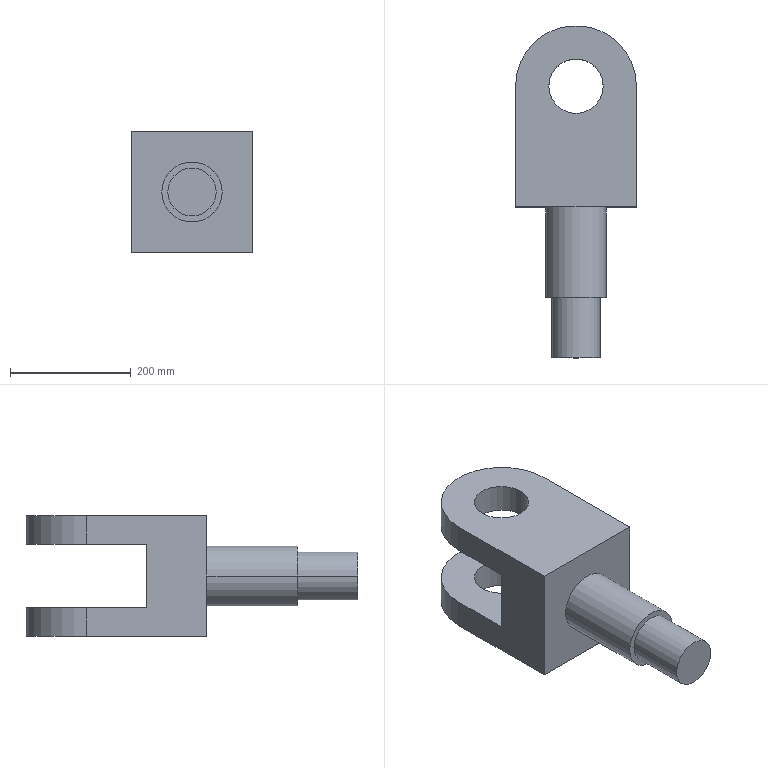Part | SolidWorks | features ICE 4, Extrusion 1 | 1 solid | 20 faces | box 200 x 550 x 200 mm | volume 8468645 mm3 | cylinder 10 | plane 10 | commonest cylinder face diameters 90 x4 80 x2 100 x2 200 x2
STEP:
#1=CARTESIAN_POINT('',(80.402,-409.598,100.));
#2=VERTEX_POINT('',#1);
#3=CARTESIAN_POINT('',(0.4025,-409.598,100.));
#4=VERTEX_POINT('',#3);
#5=CARTESIAN_POINT('',(40.402,-409.598,100.));
#6=DIRECTION('',(0.,-1.,0.));
#7=DIRECTION('',(1.,0.,0.));
#8=AXIS2_PLACEMENT_3D('',#5,#6,#7);
#9=CIRCLE('',#8,40.);
#10=EDGE_CURVE('',#2,#4,#9,.T.);
#11=ORIENTED_EDGE('',*,*,#10,.F.);
#12=CARTESIAN_POINT('',(80.402,-309.598,100.));
#13=VERTEX_POINT('',#12);
#14=CARTESIAN_POINT('',(80.402,-409.598,100.));
#15=DIRECTION('',(0.,1.,0.));
#16=VECTOR('',#15,1000.);
#17=LINE('',#14,#16);
#18=EDGE_CURVE('',#2,#13,#17,.T.);
#19=ORIENTED_EDGE('',*,*,#18,.T.);
#20=CARTESIAN_POINT('',(0.4025,-309.598,100.));
#21=VERTEX_POINT('',#20);
#22=CARTESIAN_POINT('',(40.402,-309.598,100.));
#23=DIRECTION('',(0.,-1.,0.));
#24=DIRECTION('',(1.,0.,0.));
#25=AXIS2_PLACEMENT_3D('',#22,#23,#24);
#26=CIRCLE('',#25,40.);
#27=EDGE_CURVE('',#13,#21,#26,.T.);
#28=ORIENTED_EDGE('',*,*,#27,.T.);
#29=CARTESIAN_POINT('',(0.4025,-409.598,100.));
#30=DIRECTION('',(0.,1.,0.));
#31=VECTOR('',#30,1000.);
#32=LINE('',#29,#31);
#33=EDGE_CURVE('',#4,#21,#32,.T.);
#34=ORIENTED_EDGE('',*,*,#33,.F.);
#35=EDGE_LOOP('',(#11,#19,#28,#34));
#36=FACE_OUTER_BOUND('',#35,.T.);
#37=CARTESIAN_POINT('',(40.402,-409.598,100.));
#38=DIRECTION('',(0.,1.,0.));
#39=DIRECTION('',(-1.,0.,0.));
#40=AXIS2_PLACEMENT_3D('',#37,#38,#39);
#41=CYLINDRICAL_SURFACE('',#40,40.);
#42=ADVANCED_FACE('',(#36),#41,.T.);
#43=CARTESIAN_POINT('',(90.402,-309.598,100.));
#44=VERTEX_POINT('',#43);
#45=CARTESIAN_POINT('',(-9.598,-309.598,100.));
#46=VERTEX_POINT('',#45);
#47=CARTESIAN_POINT('',(40.402,-309.598,100.));
#48=DIRECTION('',(0.,-1.,0.));
#49=DIRECTION('',(1.,0.,0.));
#50=AXIS2_PLACEMENT_3D('',#47,#48,#49);
#51=CIRCLE('',#50,50.);
#52=EDGE_CURVE('',#44,#46,#51,.T.);
#53=ORIENTED_EDGE('',*,*,#52,.F.);
#54=CARTESIAN_POINT('',(90.402,-159.598,100.));
#55=VERTEX_POINT('',#54);
#56=CARTESIAN_POINT('',(90.402,-299.598,100.));
#57=DIRECTION('',(0.,1.,0.));
#58=VECTOR('',#57,1000.);
#59=LINE('',#56,#58);
#60=EDGE_CURVE('',#44,#55,#59,.T.);
#61=ORIENTED_EDGE('',*,*,#60,.T.);
#62=CARTESIAN_POINT('',(-9.598,-159.598,100.));
#63=VERTEX_POINT('',#62);
#64=CARTESIAN_POINT('',(40.402,-159.598,100.));
#65=DIRECTION('',(0.,-1.,0.));
#66=DIRECTION('',(1.,0.,0.));
#67=AXIS2_PLACEMENT_3D('',#64,#65,#66);
#68=CIRCLE('',#67,50.);
#69=EDGE_CURVE('',#55,#63,#68,.T.);
#70=ORIENTED_EDGE('',*,*,#69,.T.);
#71=CARTESIAN_POINT('',(-9.598,-299.598,100.));
#72=DIRECTION('',(0.,1.,0.));
#73=VECTOR('',#72,1000.);
#74=LINE('',#71,#73);
#75=EDGE_CURVE('',#46,#63,#74,.T.);
#76=ORIENTED_EDGE('',*,*,#75,.F.);
#77=EDGE_LOOP('',(#53,#61,#70,#76));
#78=FACE_OUTER_BOUND('',#77,.T.);
#79=CARTESIAN_POINT('',(40.402,-299.598,100.));
#80=DIRECTION('',(0.,1.,0.));
#81=DIRECTION('',(-1.,0.,0.));
#82=AXIS2_PLACEMENT_3D('',#79,#80,#81);
#83=CYLINDRICAL_SURFACE('',#82,50.);
#84=ADVANCED_FACE('',(#78),#83,.T.);
#85=CARTESIAN_POINT('',(-4.598,40.402,200.));
#86=VERTEX_POINT('',#85);
#87=CARTESIAN_POINT('',(85.402,40.402,200.));
#88=VERTEX_POINT('',#87);
#89=CARTESIAN_POINT('',(40.402,40.402,200.));
#90=DIRECTION('',(0.,0.,1.));
#91=DIRECTION('',(1.,0.,0.));
#92=AXIS2_PLACEMENT_3D('',#89,#90,#91);
#93=CIRCLE('',#92,45.);
#94=EDGE_CURVE('',#86,#88,#93,.T.);
#95=ORIENTED_EDGE('',*,*,#94,.T.);
#96=CARTESIAN_POINT('',(85.402,40.402,152.5));
#97=VERTEX_POINT('',#96);
#98=CARTESIAN_POINT('',(85.402,40.402,200.));
#99=DIRECTION('',(0.,0.,-1.));
#100=VECTOR('',#99,1000.);
#101=LINE('',#98,#100);
#102=EDGE_CURVE('',#88,#97,#101,.T.);
#103=ORIENTED_EDGE('',*,*,#102,.T.);
#104=CARTESIAN_POINT('',(-4.598,40.402,152.5));
#105=VERTEX_POINT('',#104);
#106=CARTESIAN_POINT('',(40.402,40.402,152.5));
#107=DIRECTION('',(0.,0.,1.));
#108=DIRECTION('',(0.,-1.,0.));
#109=AXIS2_PLACEMENT_3D('',#106,#107,#108);
#110=CIRCLE('',#109,45.);
#111=EDGE_CURVE('',#105,#97,#110,.T.);
#112=ORIENTED_EDGE('',*,*,#111,.F.);
#113=CARTESIAN_POINT('',(-4.598,40.402,200.));
#114=DIRECTION('',(0.,0.,-1.));
#115=VECTOR('',#114,1000.);
#116=LINE('',#113,#115);
#117=EDGE_CURVE('',#86,#105,#116,.T.);
#118=ORIENTED_EDGE('',*,*,#117,.F.);
#119=EDGE_LOOP('',(#95,#103,#112,#118));
#120=FACE_OUTER_BOUND('',#119,.T.);
#121=CARTESIAN_POINT('',(40.402,40.402,200.));
#122=DIRECTION('',(0.,0.,-1.));
#123=DIRECTION('',(-1.,0.,0.));
#124=AXIS2_PLACEMENT_3D('',#121,#122,#123);
#125=CYLINDRICAL_SURFACE('',#124,45.);
#126=ADVANCED_FACE('',(#120),#125,.F.);
#127=CARTESIAN_POINT('',(85.402,40.402,47.5));
#128=VERTEX_POINT('',#127);
#129=CARTESIAN_POINT('',(-4.598,40.402,47.5));
#130=VERTEX_POINT('',#129);
#131=CARTESIAN_POINT('',(40.402,40.402,47.5));
#132=DIRECTION('',(0.,0.,-1.));
#133=DIRECTION('',(0.,1.,0.));
#134=AXIS2_PLACEMENT_3D('',#131,#132,#133);
#135=CIRCLE('',#134,45.);
#136=EDGE_CURVE('',#128,#130,#135,.T.);
#137=ORIENTED_EDGE('',*,*,#136,.F.);
#138=CARTESIAN_POINT('',(85.402,40.402,0.));
#139=VERTEX_POINT('',#138);
#140=CARTESIAN_POINT('',(85.402,40.402,200.));
#141=DIRECTION('',(0.,0.,-1.));
#142=VECTOR('',#141,1000.);
#143=LINE('',#140,#142);
#144=EDGE_CURVE('',#128,#139,#143,.T.);
#145=ORIENTED_EDGE('',*,*,#144,.T.);
#146=CARTESIAN_POINT('',(-4.598,40.402,0.));
#147=VERTEX_POINT('',#146);
#148=CARTESIAN_POINT('',(40.402,40.402,0.));
#149=DIRECTION('',(0.,0.,1.));
#150=DIRECTION('',(1.,0.,0.));
#151=AXIS2_PLACEMENT_3D('',#148,#149,#150);
#152=CIRCLE('',#151,45.);
#153=EDGE_CURVE('',#147,#139,#152,.T.);
#154=ORIENTED_EDGE('',*,*,#153,.F.);
#155=CARTESIAN_POINT('',(-4.598,40.402,200.));
#156=DIRECTION('',(0.,0.,-1.));
#157=VECTOR('',#156,1000.);
#158=LINE('',#155,#157);
#159=EDGE_CURVE('',#130,#147,#158,.T.);
#160=ORIENTED_EDGE('',*,*,#159,.F.);
#161=EDGE_LOOP('',(#137,#145,#154,#160));
#162=FACE_OUTER_BOUND('',#161,.T.);
#163=CARTESIAN_POINT('',(40.402,40.402,200.));
#164=DIRECTION('',(0.,0.,-1.));
#165=DIRECTION('',(-1.,0.,0.));
#166=AXIS2_PLACEMENT_3D('',#163,#164,#165);
#167=CYLINDRICAL_SURFACE('',#166,45.);
#168=ADVANCED_FACE('',(#162),#167,.F.);
#169=CARTESIAN_POINT('',(-59.598,40.402,47.5));
#170=VERTEX_POINT('',#169);
#171=CARTESIAN_POINT('',(-59.598,40.402,0.));
#172=VERTEX_POINT('',#171);
#173=CARTESIAN_POINT('',(-59.598,40.402,200.));
#174=DIRECTION('',(0.,0.,-1.));
#175=VECTOR('',#174,1000.);
#176=LINE('',#173,#175);
#177=EDGE_CURVE('',#170,#172,#176,.T.);
#178=ORIENTED_EDGE('',*,*,#177,.F.);
#179=CARTESIAN_POINT('',(140.402,40.402,47.5));
#180=VERTEX_POINT('',#179);
#181=CARTESIAN_POINT('',(40.402,40.402,47.5));
#182=DIRECTION('',(0.,0.,-1.));
#183=DIRECTION('',(0.,1.,0.));
#184=AXIS2_PLACEMENT_3D('',#181,#182,#183);
#185=CIRCLE('',#184,100.);
#186=EDGE_CURVE('',#170,#180,#185,.T.);
#187=ORIENTED_EDGE('',*,*,#186,.T.);
#188=CARTESIAN_POINT('',(140.402,40.402,0.));
#189=VERTEX_POINT('',#188);
#190=CARTESIAN_POINT('',(140.402,40.402,200.));
#191=DIRECTION('',(0.,0.,-1.));
#192=VECTOR('',#191,1000.);
#193=LINE('',#190,#192);
#194=EDGE_CURVE('',#180,#189,#193,.T.);
#195=ORIENTED_EDGE('',*,*,#194,.T.);
#196=CARTESIAN_POINT('',(40.402,40.402,0.));
#197=DIRECTION('',(0.,0.,1.));
#198=DIRECTION('',(1.,0.,0.));
#199=AXIS2_PLACEMENT_3D('',#196,#197,#198);
#200=CIRCLE('',#199,100.);
#201=EDGE_CURVE('',#189,#172,#200,.T.);
#202=ORIENTED_EDGE('',*,*,#201,.T.);
#203=EDGE_LOOP('',(#178,#187,#195,#202));
#204=FACE_OUTER_BOUND('',#203,.T.);
#205=CARTESIAN_POINT('',(40.402,40.402,200.));
#206=DIRECTION('',(0.,0.,-1.));
#207=DIRECTION('',(-1.,0.,0.));
#208=AXIS2_PLACEMENT_3D('',#205,#206,#207);
#209=CYLINDRICAL_SURFACE('',#208,100.);
#210=ADVANCED_FACE('',(#204),#209,.T.);
#211=ORIENTED_EDGE('',*,*,#144,.F.);
#212=CARTESIAN_POINT('',(40.402,40.402,47.5));
#213=DIRECTION('',(0.,0.,-1.));
#214=DIRECTION('',(0.,1.,0.));
#215=AXIS2_PLACEMENT_3D('',#212,#213,#214);
#216=CIRCLE('',#215,45.);
#217=EDGE_CURVE('',#130,#128,#216,.T.);
#218=ORIENTED_EDGE('',*,*,#217,.F.);
#219=ORIENTED_EDGE('',*,*,#159,.T.);
#220=CARTESIAN_POINT('',(40.402,40.402,0.));
#221=DIRECTION('',(0.,0.,1.));
#222=DIRECTION('',(1.,0.,0.));
#223=AXIS2_PLACEMENT_3D('',#220,#221,#222);
#224=CIRCLE('',#223,45.);
#225=EDGE_CURVE('',#139,#147,#224,.T.);
#226=ORIENTED_EDGE('',*,*,#225,.F.);
#227=EDGE_LOOP('',(#211,#218,#219,#226));
#228=FACE_OUTER_BOUND('',#227,.T.);
#229=CARTESIAN_POINT('',(40.402,40.402,200.));
#230=DIRECTION('',(0.,0.,-1.));
#231=DIRECTION('',(-1.,0.,0.));
#232=AXIS2_PLACEMENT_3D('',#229,#230,#231);
#233=CYLINDRICAL_SURFACE('',#232,45.);
#234=ADVANCED_FACE('',(#228),#233,.F.);
#235=CARTESIAN_POINT('',(140.402,40.402,200.));
#236=VERTEX_POINT('',#235);
#237=CARTESIAN_POINT('',(-59.598,40.402,200.));
#238=VERTEX_POINT('',#237);
#239=CARTESIAN_POINT('',(40.402,40.402,200.));
#240=DIRECTION('',(0.,0.,1.));
#241=DIRECTION('',(1.,0.,0.));
#242=AXIS2_PLACEMENT_3D('',#239,#240,#241);
#243=CIRCLE('',#242,100.);
#244=EDGE_CURVE('',#236,#238,#243,.T.);
#245=ORIENTED_EDGE('',*,*,#244,.T.);
#246=CARTESIAN_POINT('',(-59.598,-159.598,200.));
#247=VERTEX_POINT('',#246);
#248=CARTESIAN_POINT('',(-59.598,-159.598,200.));
#249=DIRECTION('',(0.,-1.,0.));
#250=VECTOR('',#249,1000.);
#251=LINE('',#248,#250);
#252=EDGE_CURVE('',#238,#247,#251,.T.);
#253=ORIENTED_EDGE('',*,*,#252,.T.);
#254=CARTESIAN_POINT('',(140.402,-159.598,200.));
#255=VERTEX_POINT('',#254);
#256=CARTESIAN_POINT('',(140.402,-159.598,200.));
#257=DIRECTION('',(1.,0.,0.));
#258=VECTOR('',#257,1000.);
#259=LINE('',#256,#258);
#260=EDGE_CURVE('',#247,#255,#259,.T.);
#261=ORIENTED_EDGE('',*,*,#260,.T.);
#262=CARTESIAN_POINT('',(140.402,-159.598,200.));
#263=DIRECTION('',(0.,1.,0.));
#264=VECTOR('',#263,1000.);
#265=LINE('',#262,#264);
#266=EDGE_CURVE('',#255,#236,#265,.T.);
#267=ORIENTED_EDGE('',*,*,#266,.T.);
#268=EDGE_LOOP('',(#245,#253,#261,#267));
#269=FACE_OUTER_BOUND('',#268,.T.);
#270=ORIENTED_EDGE('',*,*,#94,.F.);
#271=CARTESIAN_POINT('',(40.402,40.402,200.));
#272=DIRECTION('',(0.,0.,1.));
#273=DIRECTION('',(1.,0.,0.));
#274=AXIS2_PLACEMENT_3D('',#271,#272,#273);
#275=CIRCLE('',#274,45.);
#276=EDGE_CURVE('',#88,#86,#275,.T.);
#277=ORIENTED_EDGE('',*,*,#276,.F.);
#278=EDGE_LOOP('',(#270,#277));
#279=FACE_BOUND('',#278,.T.);
#280=CARTESIAN_POINT('',(40.402,40.402,200.));
#281=DIRECTION('',(0.,0.,1.));
#282=DIRECTION('',(1.,0.,0.));
#283=AXIS2_PLACEMENT_3D('',#280,#281,#282);
#284=PLANE('',#283);
#285=ADVANCED_FACE('',(#269,#279),#284,.T.);
#286=ORIENTED_EDGE('',*,*,#201,.F.);
#287=CARTESIAN_POINT('',(140.402,-159.598,0.));
#288=VERTEX_POINT('',#287);
#289=CARTESIAN_POINT('',(140.402,-159.598,0.));
#290=DIRECTION('',(0.,1.,0.));
#291=VECTOR('',#290,1000.);
#292=LINE('',#289,#291);
#293=EDGE_CURVE('',#288,#189,#292,.T.);
#294=ORIENTED_EDGE('',*,*,#293,.F.);
#295=CARTESIAN_POINT('',(-59.598,-159.598,0.));
#296=VERTEX_POINT('',#295);
#297=CARTESIAN_POINT('',(140.402,-159.598,0.));
#298=DIRECTION('',(1.,0.,0.));
#299=VECTOR('',#298,1000.);
#300=LINE('',#297,#299);
#301=EDGE_CURVE('',#296,#288,#300,.T.);
#302=ORIENTED_EDGE('',*,*,#301,.F.);
#303=CARTESIAN_POINT('',(-59.598,-159.598,0.));
#304=DIRECTION('',(0.,-1.,0.));
#305=VECTOR('',#304,1000.);
#306=LINE('',#303,#305);
#307=EDGE_CURVE('',#172,#296,#306,.T.);
#308=ORIENTED_EDGE('',*,*,#307,.F.);
#309=EDGE_LOOP('',(#286,#294,#302,#308));
#310=FACE_OUTER_BOUND('',#309,.T.);
#311=ORIENTED_EDGE('',*,*,#153,.T.);
#312=ORIENTED_EDGE('',*,*,#225,.T.);
#313=EDGE_LOOP('',(#311,#312));
#314=FACE_BOUND('',#313,.T.);
#315=CARTESIAN_POINT('',(40.402,40.402,0.));
#316=DIRECTION('',(0.,0.,1.));
#317=DIRECTION('',(1.,0.,0.));
#318=AXIS2_PLACEMENT_3D('',#315,#316,#317);
#319=PLANE('',#318);
#320=ADVANCED_FACE('',(#310,#314),#319,.F.);
#321=CARTESIAN_POINT('',(140.402,40.402,152.5));
#322=VERTEX_POINT('',#321);
#323=CARTESIAN_POINT('',(140.402,40.402,200.));
#324=DIRECTION('',(0.,0.,-1.));
#325=VECTOR('',#324,1000.);
#326=LINE('',#323,#325);
#327=EDGE_CURVE('',#236,#322,#326,.T.);
#328=ORIENTED_EDGE('',*,*,#327,.T.);
#329=CARTESIAN_POINT('',(-59.598,40.402,152.5));
#330=VERTEX_POINT('',#329);
#331=CARTESIAN_POINT('',(40.402,40.402,152.5));
#332=DIRECTION('',(0.,0.,1.));
#333=DIRECTION('',(0.,-1.,0.));
#334=AXIS2_PLACEMENT_3D('',#331,#332,#333);
#335=CIRCLE('',#334,100.);
#336=EDGE_CURVE('',#322,#330,#335,.T.);
#337=ORIENTED_EDGE('',*,*,#336,.T.);
#338=CARTESIAN_POINT('',(-59.598,40.402,200.));
#339=DIRECTION('',(0.,0.,-1.));
#340=VECTOR('',#339,1000.);
#341=LINE('',#338,#340);
#342=EDGE_CURVE('',#238,#330,#341,.T.);
#343=ORIENTED_EDGE('',*,*,#342,.F.);
#344=ORIENTED_EDGE('',*,*,#244,.F.);
#345=EDGE_LOOP('',(#328,#337,#343,#344));
#346=FACE_OUTER_BOUND('',#345,.T.);
#347=CARTESIAN_POINT('',(40.402,40.402,200.));
#348=DIRECTION('',(0.,0.,-1.));
#349=DIRECTION('',(-1.,0.,0.));
#350=AXIS2_PLACEMENT_3D('',#347,#348,#349);
#351=CYLINDRICAL_SURFACE('',#350,100.);
#352=ADVANCED_FACE('',(#346),#351,.T.);
#353=CARTESIAN_POINT('',(-59.598,-59.598,152.5));
#354=VERTEX_POINT('',#353);
#355=CARTESIAN_POINT('',(-59.598,-59.598,47.5));
#356=VERTEX_POINT('',#355);
#357=CARTESIAN_POINT('',(-59.598,-59.598,152.5));
#358=DIRECTION('',(0.,0.,-1.));
#359=VECTOR('',#358,1000.);
#360=LINE('',#357,#359);
#361=EDGE_CURVE('',#354,#356,#360,.T.);
#362=ORIENTED_EDGE('',*,*,#361,.T.);
#363=CARTESIAN_POINT('',(-59.598,258.452,47.5));
#364=DIRECTION('',(0.,1.,0.));
#365=VECTOR('',#364,1000.);
#366=LINE('',#363,#365);
#367=EDGE_CURVE('',#356,#170,#366,.T.);
#368=ORIENTED_EDGE('',*,*,#367,.T.);
#369=ORIENTED_EDGE('',*,*,#177,.T.);
#370=ORIENTED_EDGE('',*,*,#307,.T.);
#371=CARTESIAN_POINT('',(-59.598,-159.598,200.));
#372=DIRECTION('',(0.,0.,-1.));
#373=VECTOR('',#372,1000.);
#374=LINE('',#371,#373);
#375=EDGE_CURVE('',#247,#296,#374,.T.);
#376=ORIENTED_EDGE('',*,*,#375,.F.);
#377=ORIENTED_EDGE('',*,*,#252,.F.);
#378=ORIENTED_EDGE('',*,*,#342,.T.);
#379=CARTESIAN_POINT('',(-59.598,258.452,152.5));
#380=DIRECTION('',(0.,-1.,0.));
#381=VECTOR('',#380,1000.);
#382=LINE('',#379,#381);
#383=EDGE_CURVE('',#330,#354,#382,.T.);
#384=ORIENTED_EDGE('',*,*,#383,.T.);
#385=EDGE_LOOP('',(#362,#368,#369,#370,#376,#377,#378,#384));
#386=FACE_OUTER_BOUND('',#385,.T.);
#387=CARTESIAN_POINT('',(-59.598,-159.598,200.));
#388=DIRECTION('',(1.,0.,0.));
#389=DIRECTION('',(0.,1.,0.));
#390=AXIS2_PLACEMENT_3D('',#387,#388,#389);
#391=PLANE('',#390);
#392=ADVANCED_FACE('',(#386),#391,.F.);
#393=CARTESIAN_POINT('',(40.402,-159.598,100.));
#394=DIRECTION('',(0.,-1.,0.));
#395=DIRECTION('',(1.,0.,0.));
#396=AXIS2_PLACEMENT_3D('',#393,#394,#395);
#397=CIRCLE('',#396,50.);
#398=EDGE_CURVE('',#63,#55,#397,.T.);
#399=ORIENTED_EDGE('',*,*,#398,.F.);
#400=ORIENTED_EDGE('',*,*,#69,.F.);
#401=EDGE_LOOP('',(#399,#400));
#402=FACE_BOUND('',#401,.T.);
#403=ORIENTED_EDGE('',*,*,#301,.T.);
#404=CARTESIAN_POINT('',(140.402,-159.598,200.));
#405=DIRECTION('',(0.,0.,-1.));
#406=VECTOR('',#405,1000.);
#407=LINE('',#404,#406);
#408=EDGE_CURVE('',#255,#288,#407,.T.);
#409=ORIENTED_EDGE('',*,*,#408,.F.);
#410=ORIENTED_EDGE('',*,*,#260,.F.);
#411=ORIENTED_EDGE('',*,*,#375,.T.);
#412=EDGE_LOOP('',(#403,#409,#410,#411));
#413=FACE_OUTER_BOUND('',#412,.T.);
#414=CARTESIAN_POINT('',(140.402,-159.598,200.));
#415=DIRECTION('',(0.,1.,0.));
#416=DIRECTION('',(-1.,0.,0.));
#417=AXIS2_PLACEMENT_3D('',#414,#415,#416);
#418=PLANE('',#417);
#419=ADVANCED_FACE('',(#402,#413),#418,.F.);
#420=ORIENTED_EDGE('',*,*,#194,.F.);
#421=CARTESIAN_POINT('',(140.402,-59.598,47.5));
#422=VERTEX_POINT('',#421);
#423=CARTESIAN_POINT('',(140.402,258.452,47.5));
#424=DIRECTION('',(0.,1.,0.));
#425=VECTOR('',#424,1000.);
#426=LINE('',#423,#425);
#427=EDGE_CURVE('',#422,#180,#426,.T.);
#428=ORIENTED_EDGE('',*,*,#427,.F.);
#429=CARTESIAN_POINT('',(140.402,-59.598,152.5));
#430=VERTEX_POINT('',#429);
#431=CARTESIAN_POINT('',(140.402,-59.598,152.5));
#432=DIRECTION('',(0.,0.,-1.));
#433=VECTOR('',#432,1000.);
#434=LINE('',#431,#433);
#435=EDGE_CURVE('',#430,#422,#434,.T.);
#436=ORIENTED_EDGE('',*,*,#435,.F.);
#437=CARTESIAN_POINT('',(140.402,258.452,152.5));
#438=DIRECTION('',(0.,-1.,0.));
#439=VECTOR('',#438,1000.);
#440=LINE('',#437,#439);
#441=EDGE_CURVE('',#322,#430,#440,.T.);
#442=ORIENTED_EDGE('',*,*,#441,.F.);
#443=ORIENTED_EDGE('',*,*,#327,.F.);
#444=ORIENTED_EDGE('',*,*,#266,.F.);
#445=ORIENTED_EDGE('',*,*,#408,.T.);
#446=ORIENTED_EDGE('',*,*,#293,.T.);
#447=EDGE_LOOP('',(#420,#428,#436,#442,#443,#444,#445,#446));
#448=FACE_OUTER_BOUND('',#447,.T.);
#449=CARTESIAN_POINT('',(140.402,-159.598,200.));
#450=DIRECTION('',(-1.,0.,0.));
#451=DIRECTION('',(0.,0.,1.));
#452=AXIS2_PLACEMENT_3D('',#449,#450,#451);
#453=PLANE('',#452);
#454=ADVANCED_FACE('',(#448),#453,.F.);
#455=ORIENTED_EDGE('',*,*,#102,.F.);
#456=ORIENTED_EDGE('',*,*,#276,.T.);
#457=ORIENTED_EDGE('',*,*,#117,.T.);
#458=CARTESIAN_POINT('',(40.402,40.402,152.5));
#459=DIRECTION('',(0.,0.,1.));
#460=DIRECTION('',(0.,-1.,0.));
#461=AXIS2_PLACEMENT_3D('',#458,#459,#460);
#462=CIRCLE('',#461,45.);
#463=EDGE_CURVE('',#97,#105,#462,.T.);
#464=ORIENTED_EDGE('',*,*,#463,.F.);
#465=EDGE_LOOP('',(#455,#456,#457,#464));
#466=FACE_OUTER_BOUND('',#465,.T.);
#467=CARTESIAN_POINT('',(40.402,40.402,200.));
#468=DIRECTION('',(0.,0.,-1.));
#469=DIRECTION('',(-1.,0.,0.));
#470=AXIS2_PLACEMENT_3D('',#467,#468,#469);
#471=CYLINDRICAL_SURFACE('',#470,45.);
#472=ADVANCED_FACE('',(#466),#471,.F.);
#473=ORIENTED_EDGE('',*,*,#217,.T.);
#474=ORIENTED_EDGE('',*,*,#136,.T.);
#475=EDGE_LOOP('',(#473,#474));
#476=FACE_BOUND('',#475,.T.);
#477=ORIENTED_EDGE('',*,*,#367,.F.);
#478=CARTESIAN_POINT('',(-59.598,-59.598,47.5));
#479=DIRECTION('',(1.,0.,0.));
#480=VECTOR('',#479,1000.);
#481=LINE('',#478,#480);
#482=EDGE_CURVE('',#356,#422,#481,.T.);
#483=ORIENTED_EDGE('',*,*,#482,.T.);
#484=ORIENTED_EDGE('',*,*,#427,.T.);
#485=ORIENTED_EDGE('',*,*,#186,.F.);
#486=EDGE_LOOP('',(#477,#483,#484,#485));
#487=FACE_OUTER_BOUND('',#486,.T.);
#488=CARTESIAN_POINT('',(-59.598,258.452,47.5));
#489=DIRECTION('',(0.,0.,-1.));
#490=DIRECTION('',(0.,1.,0.));
#491=AXIS2_PLACEMENT_3D('',#488,#489,#490);
#492=PLANE('',#491);
#493=ADVANCED_FACE('',(#476,#487),#492,.F.);
#494=ORIENTED_EDGE('',*,*,#111,.T.);
#495=ORIENTED_EDGE('',*,*,#463,.T.);
#496=EDGE_LOOP('',(#494,#495));
#497=FACE_BOUND('',#496,.T.);
#498=ORIENTED_EDGE('',*,*,#441,.T.);
#499=CARTESIAN_POINT('',(-59.598,-59.598,152.5));
#500=DIRECTION('',(1.,0.,0.));
#501=VECTOR('',#500,1000.);
#502=LINE('',#499,#501);
#503=EDGE_CURVE('',#354,#430,#502,.T.);
#504=ORIENTED_EDGE('',*,*,#503,.F.);
#505=ORIENTED_EDGE('',*,*,#383,.F.);
#506=ORIENTED_EDGE('',*,*,#336,.F.);
#507=EDGE_LOOP('',(#498,#504,#505,#506));
#508=FACE_OUTER_BOUND('',#507,.T.);
#509=CARTESIAN_POINT('',(-59.598,258.452,152.5));
#510=DIRECTION('',(0.,0.,1.));
#511=DIRECTION('',(0.,-1.,0.));
#512=AXIS2_PLACEMENT_3D('',#509,#510,#511);
#513=PLANE('',#512);
#514=ADVANCED_FACE('',(#497,#508),#513,.F.);
#515=ORIENTED_EDGE('',*,*,#435,.T.);
#516=ORIENTED_EDGE('',*,*,#482,.F.);
#517=ORIENTED_EDGE('',*,*,#361,.F.);
#518=ORIENTED_EDGE('',*,*,#503,.T.);
#519=EDGE_LOOP('',(#515,#516,#517,#518));
#520=FACE_OUTER_BOUND('',#519,.T.);
#521=CARTESIAN_POINT('',(-59.598,-59.598,152.5));
#522=DIRECTION('',(0.,-1.,0.));
#523=DIRECTION('',(0.,0.,-1.));
#524=AXIS2_PLACEMENT_3D('',#521,#522,#523);
#525=PLANE('',#524);
#526=ADVANCED_FACE('',(#520),#525,.F.);
#527=ORIENTED_EDGE('',*,*,#60,.F.);
#528=CARTESIAN_POINT('',(40.402,-309.598,100.));
#529=DIRECTION('',(0.,-1.,0.));
#530=DIRECTION('',(1.,0.,0.));
#531=AXIS2_PLACEMENT_3D('',#528,#529,#530);
#532=CIRCLE('',#531,50.);
#533=EDGE_CURVE('',#46,#44,#532,.T.);
#534=ORIENTED_EDGE('',*,*,#533,.F.);
#535=ORIENTED_EDGE('',*,*,#75,.T.);
#536=ORIENTED_EDGE('',*,*,#398,.T.);
#537=EDGE_LOOP('',(#527,#534,#535,#536));
#538=FACE_OUTER_BOUND('',#537,.T.);
#539=CARTESIAN_POINT('',(40.402,-299.598,100.));
#540=DIRECTION('',(0.,1.,0.));
#541=DIRECTION('',(-1.,0.,0.));
#542=AXIS2_PLACEMENT_3D('',#539,#540,#541);
#543=CYLINDRICAL_SURFACE('',#542,50.);
#544=ADVANCED_FACE('',(#538),#543,.T.);
#545=CARTESIAN_POINT('',(40.402,-309.598,100.));
#546=DIRECTION('',(0.,-1.,0.));
#547=DIRECTION('',(1.,0.,0.));
#548=AXIS2_PLACEMENT_3D('',#545,#546,#547);
#549=CIRCLE('',#548,40.);
#550=EDGE_CURVE('',#21,#13,#549,.T.);
#551=ORIENTED_EDGE('',*,*,#550,.F.);
#552=ORIENTED_EDGE('',*,*,#27,.F.);
#553=EDGE_LOOP('',(#551,#552));
#554=FACE_BOUND('',#553,.T.);
#555=ORIENTED_EDGE('',*,*,#533,.T.);
#556=ORIENTED_EDGE('',*,*,#52,.T.);
#557=EDGE_LOOP('',(#555,#556));
#558=FACE_OUTER_BOUND('',#557,.T.);
#559=CARTESIAN_POINT('',(40.402,-309.598,100.));
#560=DIRECTION('',(0.,-1.,0.));
#561=DIRECTION('',(1.,0.,0.));
#562=AXIS2_PLACEMENT_3D('',#559,#560,#561);
#563=PLANE('',#562);
#564=ADVANCED_FACE('',(#554,#558),#563,.T.);
#565=ORIENTED_EDGE('',*,*,#18,.F.);
#566=CARTESIAN_POINT('',(40.402,-409.598,100.));
#567=DIRECTION('',(0.,-1.,0.));
#568=DIRECTION('',(1.,0.,0.));
#569=AXIS2_PLACEMENT_3D('',#566,#567,#568);
#570=CIRCLE('',#569,40.);
#571=EDGE_CURVE('',#4,#2,#570,.T.);
#572=ORIENTED_EDGE('',*,*,#571,.F.);
#573=ORIENTED_EDGE('',*,*,#33,.T.);
#574=ORIENTED_EDGE('',*,*,#550,.T.);
#575=EDGE_LOOP('',(#565,#572,#573,#574));
#576=FACE_OUTER_BOUND('',#575,.T.);
#577=CARTESIAN_POINT('',(40.402,-409.598,100.));
#578=DIRECTION('',(0.,1.,0.));
#579=DIRECTION('',(-1.,0.,0.));
#580=AXIS2_PLACEMENT_3D('',#577,#578,#579);
#581=CYLINDRICAL_SURFACE('',#580,40.);
#582=ADVANCED_FACE('',(#576),#581,.T.);
#583=ORIENTED_EDGE('',*,*,#571,.T.);
#584=ORIENTED_EDGE('',*,*,#10,.T.);
#585=EDGE_LOOP('',(#583,#584));
#586=FACE_OUTER_BOUND('',#585,.T.);
#587=CARTESIAN_POINT('',(40.402,-409.598,100.));
#588=DIRECTION('',(0.,-1.,0.));
#589=DIRECTION('',(1.,0.,0.));
#590=AXIS2_PLACEMENT_3D('',#587,#588,#589);
#591=PLANE('',#590);
#592=ADVANCED_FACE('',(#586),#591,.T.);
#593=CLOSED_SHELL('',(#42,#84,#126,#168,#210,#234,#285,#320,#352,#392,#419,#454,#472,#493,#514,#526,#544,#564,#582,#592));
#594=MANIFOLD_SOLID_BREP('',#593);
#595=CARTESIAN_POINT('',(0.,0.,0.));
#596=DIRECTION('',(0.,0.,1.));
#597=DIRECTION('',(1.,0.,0.));
#598=AXIS2_PLACEMENT_3D('',#595,#596,#597);
#599=(LENGTH_UNIT()NAMED_UNIT(*)SI_UNIT(.MILLI.,.METRE.));
#600=UNCERTAINTY_MEASURE_WITH_UNIT(LENGTH_MEASURE(0.00001),#599,'','');
#601=(NAMED_UNIT(*)PLANE_ANGLE_UNIT()SI_UNIT($,.RADIAN.));
#602=(NAMED_UNIT(*)SI_UNIT($,.STERADIAN.)SOLID_ANGLE_UNIT());
#603=(GEOMETRIC_REPRESENTATION_CONTEXT(3)GLOBAL_UNCERTAINTY_ASSIGNED_CONTEXT((#600))GLOBAL_UNIT_ASSIGNED_CONTEXT((#599,#601,#602))REPRESENTATION_CONTEXT('',''));
#604=ADVANCED_BREP_SHAPE_REPRESENTATION('',(#594,#598),#603);